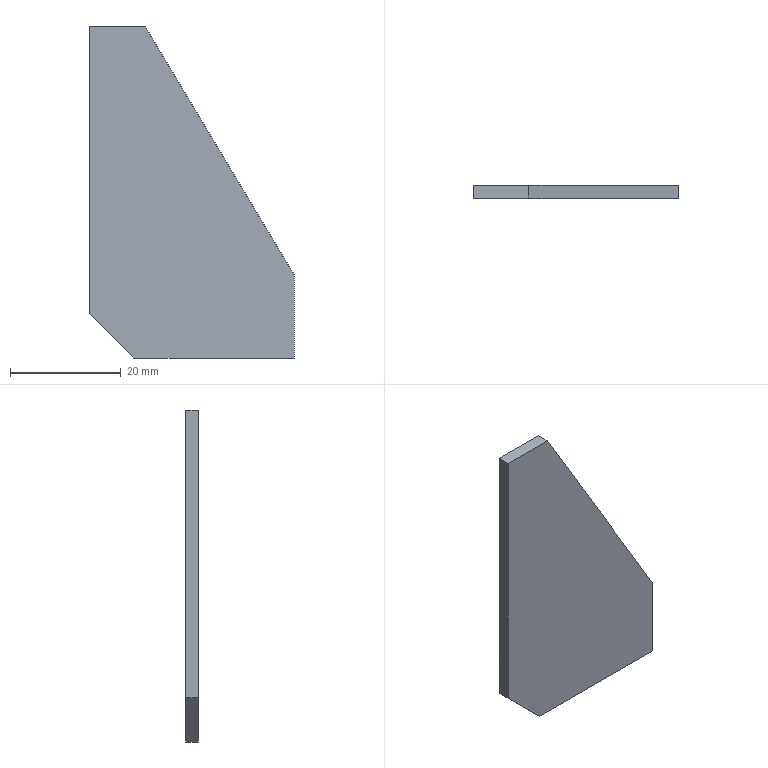Part | SolidWorks | features FlatPattern 1, SMBaseFlange 1, SheetMetal 1 | 1 solid | 8 faces | box 37 x 2.3 x 60 mm | volume 3635 mm3 | plane 8
STEP:
#1=CARTESIAN_POINT('',(0.,0.,0.));
#2=VERTEX_POINT('',#1);
#3=CARTESIAN_POINT('',(10.,0.,0.));
#4=VERTEX_POINT('',#3);
#5=CARTESIAN_POINT('',(10.,0.,0.));
#6=DIRECTION('',(1.,0.,0.));
#7=VECTOR('',#6,1000.);
#8=LINE('',#5,#7);
#9=EDGE_CURVE('',#2,#4,#8,.T.);
#10=ORIENTED_EDGE('',*,*,#9,.F.);
#11=CARTESIAN_POINT('',(0.,-2.3,0.));
#12=VERTEX_POINT('',#11);
#13=CARTESIAN_POINT('',(0.,-2.3,0.));
#14=DIRECTION('',(0.,1.,0.));
#15=VECTOR('',#14,1000.);
#16=LINE('',#13,#15);
#17=EDGE_CURVE('',#12,#2,#16,.T.);
#18=ORIENTED_EDGE('',*,*,#17,.F.);
#19=CARTESIAN_POINT('',(10.,-2.3,0.));
#20=VERTEX_POINT('',#19);
#21=CARTESIAN_POINT('',(10.,-2.3,0.));
#22=DIRECTION('',(1.,0.,0.));
#23=VECTOR('',#22,1000.);
#24=LINE('',#21,#23);
#25=EDGE_CURVE('',#12,#20,#24,.T.);
#26=ORIENTED_EDGE('',*,*,#25,.T.);
#27=CARTESIAN_POINT('',(10.,-2.3,0.));
#28=DIRECTION('',(0.,1.,0.));
#29=VECTOR('',#28,1000.);
#30=LINE('',#27,#29);
#31=EDGE_CURVE('',#20,#4,#30,.T.);
#32=ORIENTED_EDGE('',*,*,#31,.T.);
#33=EDGE_LOOP('',(#10,#18,#26,#32));
#34=FACE_OUTER_BOUND('',#33,.T.);
#35=CARTESIAN_POINT('',(10.,-2.3,0.));
#36=DIRECTION('',(0.,0.,1.));
#37=DIRECTION('',(1.,0.,0.));
#38=AXIS2_PLACEMENT_3D('',#35,#36,#37);
#39=PLANE('',#38);
#40=ADVANCED_FACE('',(#34),#39,.T.);
#41=CARTESIAN_POINT('',(0.,0.,-52.));
#42=VERTEX_POINT('',#41);
#43=CARTESIAN_POINT('',(0.,0.,0.));
#44=DIRECTION('',(0.,0.,1.));
#45=VECTOR('',#44,1000.);
#46=LINE('',#43,#45);
#47=EDGE_CURVE('',#42,#2,#46,.T.);
#48=ORIENTED_EDGE('',*,*,#47,.F.);
#49=CARTESIAN_POINT('',(0.,-2.3,-52.));
#50=VERTEX_POINT('',#49);
#51=CARTESIAN_POINT('',(0.,-2.3,-52.));
#52=DIRECTION('',(0.,1.,0.));
#53=VECTOR('',#52,1000.);
#54=LINE('',#51,#53);
#55=EDGE_CURVE('',#50,#42,#54,.T.);
#56=ORIENTED_EDGE('',*,*,#55,.F.);
#57=CARTESIAN_POINT('',(0.,-2.3,0.));
#58=DIRECTION('',(0.,0.,1.));
#59=VECTOR('',#58,1000.);
#60=LINE('',#57,#59);
#61=EDGE_CURVE('',#50,#12,#60,.T.);
#62=ORIENTED_EDGE('',*,*,#61,.T.);
#63=ORIENTED_EDGE('',*,*,#17,.T.);
#64=EDGE_LOOP('',(#48,#56,#62,#63));
#65=FACE_OUTER_BOUND('',#64,.T.);
#66=CARTESIAN_POINT('',(0.,-2.3,0.));
#67=DIRECTION('',(-1.,0.,0.));
#68=DIRECTION('',(0.,0.,1.));
#69=AXIS2_PLACEMENT_3D('',#66,#67,#68);
#70=PLANE('',#69);
#71=ADVANCED_FACE('',(#65),#70,.T.);
#72=CARTESIAN_POINT('',(8.,0.,-60.));
#73=VERTEX_POINT('',#72);
#74=CARTESIAN_POINT('',(0.,0.,-52.));
#75=DIRECTION('',(-0.7071,0.,0.7071));
#76=VECTOR('',#75,1000.);
#77=LINE('',#74,#76);
#78=EDGE_CURVE('',#73,#42,#77,.T.);
#79=ORIENTED_EDGE('',*,*,#78,.F.);
#80=CARTESIAN_POINT('',(8.,-2.3,-60.));
#81=VERTEX_POINT('',#80);
#82=CARTESIAN_POINT('',(8.,-2.3,-60.));
#83=DIRECTION('',(0.,1.,0.));
#84=VECTOR('',#83,1000.);
#85=LINE('',#82,#84);
#86=EDGE_CURVE('',#81,#73,#85,.T.);
#87=ORIENTED_EDGE('',*,*,#86,.F.);
#88=CARTESIAN_POINT('',(0.,-2.3,-52.));
#89=DIRECTION('',(-0.7071,0.,0.7071));
#90=VECTOR('',#89,1000.);
#91=LINE('',#88,#90);
#92=EDGE_CURVE('',#81,#50,#91,.T.);
#93=ORIENTED_EDGE('',*,*,#92,.T.);
#94=ORIENTED_EDGE('',*,*,#55,.T.);
#95=EDGE_LOOP('',(#79,#87,#93,#94));
#96=FACE_OUTER_BOUND('',#95,.T.);
#97=CARTESIAN_POINT('',(0.,-2.3,-52.));
#98=DIRECTION('',(-0.7071,0.,-0.7071));
#99=DIRECTION('',(-0.7071,0.,0.7071));
#100=AXIS2_PLACEMENT_3D('',#97,#98,#99);
#101=PLANE('',#100);
#102=ADVANCED_FACE('',(#96),#101,.T.);
#103=CARTESIAN_POINT('',(37.,0.,-60.));
#104=VERTEX_POINT('',#103);
#105=CARTESIAN_POINT('',(8.,0.,-60.));
#106=DIRECTION('',(-1.,0.,0.));
#107=VECTOR('',#106,1000.);
#108=LINE('',#105,#107);
#109=EDGE_CURVE('',#104,#73,#108,.T.);
#110=ORIENTED_EDGE('',*,*,#109,.F.);
#111=CARTESIAN_POINT('',(37.,-2.3,-60.));
#112=VERTEX_POINT('',#111);
#113=CARTESIAN_POINT('',(37.,-2.3,-60.));
#114=DIRECTION('',(0.,1.,0.));
#115=VECTOR('',#114,1000.);
#116=LINE('',#113,#115);
#117=EDGE_CURVE('',#112,#104,#116,.T.);
#118=ORIENTED_EDGE('',*,*,#117,.F.);
#119=CARTESIAN_POINT('',(8.,-2.3,-60.));
#120=DIRECTION('',(-1.,0.,0.));
#121=VECTOR('',#120,1000.);
#122=LINE('',#119,#121);
#123=EDGE_CURVE('',#112,#81,#122,.T.);
#124=ORIENTED_EDGE('',*,*,#123,.T.);
#125=ORIENTED_EDGE('',*,*,#86,.T.);
#126=EDGE_LOOP('',(#110,#118,#124,#125));
#127=FACE_OUTER_BOUND('',#126,.T.);
#128=CARTESIAN_POINT('',(8.,-2.3,-60.));
#129=DIRECTION('',(0.,0.,-1.));
#130=DIRECTION('',(-1.,0.,0.));
#131=AXIS2_PLACEMENT_3D('',#128,#129,#130);
#132=PLANE('',#131);
#133=ADVANCED_FACE('',(#127),#132,.T.);
#134=CARTESIAN_POINT('',(37.,0.,-45.));
#135=VERTEX_POINT('',#134);
#136=CARTESIAN_POINT('',(37.,0.,-60.));
#137=DIRECTION('',(0.,0.,-1.));
#138=VECTOR('',#137,1000.);
#139=LINE('',#136,#138);
#140=EDGE_CURVE('',#135,#104,#139,.T.);
#141=ORIENTED_EDGE('',*,*,#140,.F.);
#142=CARTESIAN_POINT('',(37.,-2.3,-45.));
#143=VERTEX_POINT('',#142);
#144=CARTESIAN_POINT('',(37.,-2.3,-45.));
#145=DIRECTION('',(0.,1.,0.));
#146=VECTOR('',#145,1000.);
#147=LINE('',#144,#146);
#148=EDGE_CURVE('',#143,#135,#147,.T.);
#149=ORIENTED_EDGE('',*,*,#148,.F.);
#150=CARTESIAN_POINT('',(37.,-2.3,-60.));
#151=DIRECTION('',(0.,0.,-1.));
#152=VECTOR('',#151,1000.);
#153=LINE('',#150,#152);
#154=EDGE_CURVE('',#143,#112,#153,.T.);
#155=ORIENTED_EDGE('',*,*,#154,.T.);
#156=ORIENTED_EDGE('',*,*,#117,.T.);
#157=EDGE_LOOP('',(#141,#149,#155,#156));
#158=FACE_OUTER_BOUND('',#157,.T.);
#159=CARTESIAN_POINT('',(37.,-2.3,-60.));
#160=DIRECTION('',(1.,0.,0.));
#161=DIRECTION('',(0.,0.,-1.));
#162=AXIS2_PLACEMENT_3D('',#159,#160,#161);
#163=PLANE('',#162);
#164=ADVANCED_FACE('',(#158),#163,.T.);
#165=CARTESIAN_POINT('',(37.,0.,-45.));
#166=DIRECTION('',(0.5145,0.,-0.8575));
#167=VECTOR('',#166,1000.);
#168=LINE('',#165,#167);
#169=EDGE_CURVE('',#4,#135,#168,.T.);
#170=ORIENTED_EDGE('',*,*,#169,.F.);
#171=ORIENTED_EDGE('',*,*,#31,.F.);
#172=CARTESIAN_POINT('',(37.,-2.3,-45.));
#173=DIRECTION('',(0.5145,0.,-0.8575));
#174=VECTOR('',#173,1000.);
#175=LINE('',#172,#174);
#176=EDGE_CURVE('',#20,#143,#175,.T.);
#177=ORIENTED_EDGE('',*,*,#176,.T.);
#178=ORIENTED_EDGE('',*,*,#148,.T.);
#179=EDGE_LOOP('',(#170,#171,#177,#178));
#180=FACE_OUTER_BOUND('',#179,.T.);
#181=CARTESIAN_POINT('',(37.,-2.3,-45.));
#182=DIRECTION('',(0.8575,0.,0.5145));
#183=DIRECTION('',(0.5145,0.,-0.8575));
#184=AXIS2_PLACEMENT_3D('',#181,#182,#183);
#185=PLANE('',#184);
#186=ADVANCED_FACE('',(#180),#185,.T.);
#187=ORIENTED_EDGE('',*,*,#25,.F.);
#188=ORIENTED_EDGE('',*,*,#61,.F.);
#189=ORIENTED_EDGE('',*,*,#92,.F.);
#190=ORIENTED_EDGE('',*,*,#123,.F.);
#191=ORIENTED_EDGE('',*,*,#154,.F.);
#192=ORIENTED_EDGE('',*,*,#176,.F.);
#193=EDGE_LOOP('',(#187,#188,#189,#190,#191,#192));
#194=FACE_OUTER_BOUND('',#193,.T.);
#195=CARTESIAN_POINT('',(0.,-2.3,0.));
#196=DIRECTION('',(0.,-1.,0.));
#197=DIRECTION('',(0.,0.,-1.));
#198=AXIS2_PLACEMENT_3D('',#195,#196,#197);
#199=PLANE('',#198);
#200=ADVANCED_FACE('',(#194),#199,.T.);
#201=ORIENTED_EDGE('',*,*,#9,.T.);
#202=ORIENTED_EDGE('',*,*,#169,.T.);
#203=ORIENTED_EDGE('',*,*,#140,.T.);
#204=ORIENTED_EDGE('',*,*,#109,.T.);
#205=ORIENTED_EDGE('',*,*,#78,.T.);
#206=ORIENTED_EDGE('',*,*,#47,.T.);
#207=EDGE_LOOP('',(#201,#202,#203,#204,#205,#206));
#208=FACE_OUTER_BOUND('',#207,.T.);
#209=CARTESIAN_POINT('',(0.,0.,0.));
#210=DIRECTION('',(0.,-1.,0.));
#211=DIRECTION('',(0.,0.,-1.));
#212=AXIS2_PLACEMENT_3D('',#209,#210,#211);
#213=PLANE('',#212);
#214=ADVANCED_FACE('',(#208),#213,.F.);
#215=CLOSED_SHELL('',(#40,#71,#102,#133,#164,#186,#200,#214));
#216=MANIFOLD_SOLID_BREP('',#215);
#217=CARTESIAN_POINT('',(0.,0.,0.));
#218=DIRECTION('',(0.,0.,1.));
#219=DIRECTION('',(1.,0.,0.));
#220=AXIS2_PLACEMENT_3D('',#217,#218,#219);
#221=(LENGTH_UNIT()NAMED_UNIT(*)SI_UNIT(.MILLI.,.METRE.));
#222=UNCERTAINTY_MEASURE_WITH_UNIT(LENGTH_MEASURE(0.00001),#221,'','');
#223=(NAMED_UNIT(*)PLANE_ANGLE_UNIT()SI_UNIT($,.RADIAN.));
#224=(NAMED_UNIT(*)SI_UNIT($,.STERADIAN.)SOLID_ANGLE_UNIT());
#225=(GEOMETRIC_REPRESENTATION_CONTEXT(3)GLOBAL_UNCERTAINTY_ASSIGNED_CONTEXT((#222))GLOBAL_UNIT_ASSIGNED_CONTEXT((#221,#223,#224))REPRESENTATION_CONTEXT('',''));
#226=ADVANCED_BREP_SHAPE_REPRESENTATION('',(#216,#220),#225);